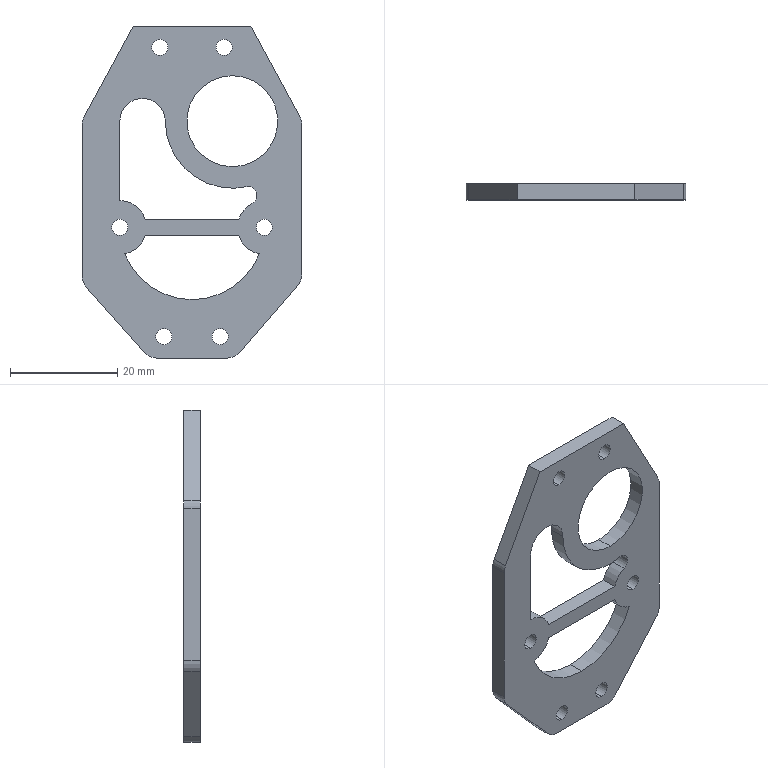Part | SolidWorks | features Extrusion 1, Fillet 1 | 1 solid | 43 faces | box 40.999 x 3 x 62 mm | volume 4212 mm3 | cylinder 30 | plane 13 | commonest cylinder face diameters 3 x12 6 x6 10 x4 17 x2 25 x2 27 x2
STEP:
#1=CARTESIAN_POINT('',(-4.98,3.,-17.786));
#2=VERTEX_POINT('',#1);
#3=CARTESIAN_POINT('',(7.52,3.,-30.28));
#4=VERTEX_POINT('',#3);
#5=CARTESIAN_POINT('',(7.52,3.,-17.78));
#6=DIRECTION('',(0.,-1.,0.));
#7=DIRECTION('',(0.,0.,1.));
#8=AXIS2_PLACEMENT_3D('',#5,#6,#7);
#9=CIRCLE('',#8,12.5);
#10=EDGE_CURVE('',#2,#4,#9,.T.);
#11=ORIENTED_EDGE('',*,*,#10,.T.);
#12=CARTESIAN_POINT('',(7.52,0.,-30.28));
#13=VERTEX_POINT('',#12);
#14=CARTESIAN_POINT('',(7.52,3.,-30.28));
#15=DIRECTION('',(0.,-1.,0.));
#16=VECTOR('',#15,1000.);
#17=LINE('',#14,#16);
#18=EDGE_CURVE('',#4,#13,#17,.T.);
#19=ORIENTED_EDGE('',*,*,#18,.T.);
#20=CARTESIAN_POINT('',(-4.98,0.,-17.786));
#21=VERTEX_POINT('',#20);
#22=CARTESIAN_POINT('',(7.52,0.,-17.78));
#23=DIRECTION('',(0.,-1.,0.));
#24=DIRECTION('',(0.,0.,1.));
#25=AXIS2_PLACEMENT_3D('',#22,#23,#24);
#26=CIRCLE('',#25,12.5);
#27=EDGE_CURVE('',#21,#13,#26,.T.);
#28=ORIENTED_EDGE('',*,*,#27,.F.);
#29=CARTESIAN_POINT('',(-4.98,3.,-17.786));
#30=DIRECTION('',(0.,-1.,0.));
#31=VECTOR('',#30,1000.);
#32=LINE('',#29,#31);
#33=EDGE_CURVE('',#2,#21,#32,.T.);
#34=ORIENTED_EDGE('',*,*,#33,.F.);
#35=EDGE_LOOP('',(#11,#19,#28,#34));
#36=FACE_OUTER_BOUND('',#35,.T.);
#37=CARTESIAN_POINT('',(7.52,3.,-17.78));
#38=DIRECTION('',(0.,-1.,0.));
#39=DIRECTION('',(0.,0.,-1.));
#40=AXIS2_PLACEMENT_3D('',#37,#38,#39);
#41=CYLINDRICAL_SURFACE('',#40,12.5);
#42=ADVANCED_FACE('',(#36),#41,.T.);
#43=CARTESIAN_POINT('',(12.574,3.,-42.519));
#44=VERTEX_POINT('',#43);
#45=CARTESIAN_POINT('',(0.,3.,-51.105));
#46=VERTEX_POINT('',#45);
#47=CARTESIAN_POINT('',(0.,3.,-37.605));
#48=DIRECTION('',(0.,1.,0.));
#49=DIRECTION('',(0.,0.,1.));
#50=AXIS2_PLACEMENT_3D('',#47,#48,#49);
#51=CIRCLE('',#50,13.5);
#52=EDGE_CURVE('',#44,#46,#51,.T.);
#53=ORIENTED_EDGE('',*,*,#52,.T.);
#54=CARTESIAN_POINT('',(0.,0.,-51.105));
#55=VERTEX_POINT('',#54);
#56=CARTESIAN_POINT('',(0.,3.,-51.105));
#57=DIRECTION('',(0.,-1.,0.));
#58=VECTOR('',#57,1000.);
#59=LINE('',#56,#58);
#60=EDGE_CURVE('',#46,#55,#59,.T.);
#61=ORIENTED_EDGE('',*,*,#60,.T.);
#62=CARTESIAN_POINT('',(12.574,0.,-42.519));
#63=VERTEX_POINT('',#62);
#64=CARTESIAN_POINT('',(0.,0.,-37.605));
#65=DIRECTION('',(0.,1.,0.));
#66=DIRECTION('',(0.,0.,1.));
#67=AXIS2_PLACEMENT_3D('',#64,#65,#66);
#68=CIRCLE('',#67,13.5);
#69=EDGE_CURVE('',#63,#55,#68,.T.);
#70=ORIENTED_EDGE('',*,*,#69,.F.);
#71=CARTESIAN_POINT('',(12.574,3.,-42.519));
#72=DIRECTION('',(0.,-1.,0.));
#73=VECTOR('',#72,1000.);
#74=LINE('',#71,#73);
#75=EDGE_CURVE('',#44,#63,#74,.T.);
#76=ORIENTED_EDGE('',*,*,#75,.F.);
#77=EDGE_LOOP('',(#53,#61,#70,#76));
#78=FACE_OUTER_BOUND('',#77,.T.);
#79=CARTESIAN_POINT('',(0.,3.,-37.605));
#80=DIRECTION('',(0.,-1.,0.));
#81=DIRECTION('',(0.,0.,-1.));
#82=AXIS2_PLACEMENT_3D('',#79,#80,#81);
#83=CYLINDRICAL_SURFACE('',#82,13.5);
#84=ADVANCED_FACE('',(#78),#83,.F.);
#85=CARTESIAN_POINT('',(13.5,3.,-39.105));
#86=VERTEX_POINT('',#85);
#87=CARTESIAN_POINT('',(13.5,3.,-36.105));
#88=VERTEX_POINT('',#87);
#89=CARTESIAN_POINT('',(13.5,3.,-37.605));
#90=DIRECTION('',(0.,1.,0.));
#91=DIRECTION('',(0.,0.,1.));
#92=AXIS2_PLACEMENT_3D('',#89,#90,#91);
#93=CIRCLE('',#92,1.5);
#94=EDGE_CURVE('',#86,#88,#93,.T.);
#95=ORIENTED_EDGE('',*,*,#94,.T.);
#96=CARTESIAN_POINT('',(13.5,0.,-36.105));
#97=VERTEX_POINT('',#96);
#98=CARTESIAN_POINT('',(13.5,3.,-36.105));
#99=DIRECTION('',(0.,-1.,0.));
#100=VECTOR('',#99,1000.);
#101=LINE('',#98,#100);
#102=EDGE_CURVE('',#88,#97,#101,.T.);
#103=ORIENTED_EDGE('',*,*,#102,.T.);
#104=CARTESIAN_POINT('',(13.5,0.,-39.105));
#105=VERTEX_POINT('',#104);
#106=CARTESIAN_POINT('',(13.5,0.,-37.605));
#107=DIRECTION('',(0.,1.,0.));
#108=DIRECTION('',(0.,0.,1.));
#109=AXIS2_PLACEMENT_3D('',#106,#107,#108);
#110=CIRCLE('',#109,1.5);
#111=EDGE_CURVE('',#105,#97,#110,.T.);
#112=ORIENTED_EDGE('',*,*,#111,.F.);
#113=CARTESIAN_POINT('',(13.5,3.,-39.105));
#114=DIRECTION('',(0.,-1.,0.));
#115=VECTOR('',#114,1000.);
#116=LINE('',#113,#115);
#117=EDGE_CURVE('',#86,#105,#116,.T.);
#118=ORIENTED_EDGE('',*,*,#117,.F.);
#119=EDGE_LOOP('',(#95,#103,#112,#118));
#120=FACE_OUTER_BOUND('',#119,.T.);
#121=CARTESIAN_POINT('',(13.5,3.,-37.605));
#122=DIRECTION('',(0.,-1.,0.));
#123=DIRECTION('',(0.,0.,-1.));
#124=AXIS2_PLACEMENT_3D('',#121,#122,#123);
#125=CYLINDRICAL_SURFACE('',#124,1.5);
#126=ADVANCED_FACE('',(#120),#125,.F.);
#127=CARTESIAN_POINT('',(-13.5,3.,-39.105));
#128=VERTEX_POINT('',#127);
#129=CARTESIAN_POINT('',(-13.5,3.,-36.105));
#130=VERTEX_POINT('',#129);
#131=CARTESIAN_POINT('',(-13.5,3.,-37.605));
#132=DIRECTION('',(0.,1.,0.));
#133=DIRECTION('',(0.,0.,1.));
#134=AXIS2_PLACEMENT_3D('',#131,#132,#133);
#135=CIRCLE('',#134,1.5);
#136=EDGE_CURVE('',#128,#130,#135,.T.);
#137=ORIENTED_EDGE('',*,*,#136,.T.);
#138=CARTESIAN_POINT('',(-13.5,0.,-36.105));
#139=VERTEX_POINT('',#138);
#140=CARTESIAN_POINT('',(-13.5,3.,-36.105));
#141=DIRECTION('',(0.,-1.,0.));
#142=VECTOR('',#141,1000.);
#143=LINE('',#140,#142);
#144=EDGE_CURVE('',#130,#139,#143,.T.);
#145=ORIENTED_EDGE('',*,*,#144,.T.);
#146=CARTESIAN_POINT('',(-13.5,0.,-39.105));
#147=VERTEX_POINT('',#146);
#148=CARTESIAN_POINT('',(-13.5,0.,-37.605));
#149=DIRECTION('',(0.,1.,0.));
#150=DIRECTION('',(0.,0.,1.));
#151=AXIS2_PLACEMENT_3D('',#148,#149,#150);
#152=CIRCLE('',#151,1.5);
#153=EDGE_CURVE('',#147,#139,#152,.T.);
#154=ORIENTED_EDGE('',*,*,#153,.F.);
#155=CARTESIAN_POINT('',(-13.5,3.,-39.105));
#156=DIRECTION('',(0.,-1.,0.));
#157=VECTOR('',#156,1000.);
#158=LINE('',#155,#157);
#159=EDGE_CURVE('',#128,#147,#158,.T.);
#160=ORIENTED_EDGE('',*,*,#159,.F.);
#161=EDGE_LOOP('',(#137,#145,#154,#160));
#162=FACE_OUTER_BOUND('',#161,.T.);
#163=CARTESIAN_POINT('',(-13.5,3.,-37.605));
#164=DIRECTION('',(0.,-1.,0.));
#165=DIRECTION('',(0.,0.,-1.));
#166=AXIS2_PLACEMENT_3D('',#163,#164,#165);
#167=CYLINDRICAL_SURFACE('',#166,1.5);
#168=ADVANCED_FACE('',(#162),#167,.F.);
#169=CARTESIAN_POINT('',(5.25,3.,-59.5));
#170=VERTEX_POINT('',#169);
#171=CARTESIAN_POINT('',(5.25,3.,-56.5));
#172=VERTEX_POINT('',#171);
#173=CARTESIAN_POINT('',(5.25,3.,-58.));
#174=DIRECTION('',(0.,1.,0.));
#175=DIRECTION('',(0.,0.,1.));
#176=AXIS2_PLACEMENT_3D('',#173,#174,#175);
#177=CIRCLE('',#176,1.5);
#178=EDGE_CURVE('',#170,#172,#177,.T.);
#179=ORIENTED_EDGE('',*,*,#178,.T.);
#180=CARTESIAN_POINT('',(5.25,0.,-56.5));
#181=VERTEX_POINT('',#180);
#182=CARTESIAN_POINT('',(5.25,3.,-56.5));
#183=DIRECTION('',(0.,-1.,0.));
#184=VECTOR('',#183,1000.);
#185=LINE('',#182,#184);
#186=EDGE_CURVE('',#172,#181,#185,.T.);
#187=ORIENTED_EDGE('',*,*,#186,.T.);
#188=CARTESIAN_POINT('',(5.25,0.,-59.5));
#189=VERTEX_POINT('',#188);
#190=CARTESIAN_POINT('',(5.25,0.,-58.));
#191=DIRECTION('',(0.,1.,0.));
#192=DIRECTION('',(0.,0.,1.));
#193=AXIS2_PLACEMENT_3D('',#190,#191,#192);
#194=CIRCLE('',#193,1.5);
#195=EDGE_CURVE('',#189,#181,#194,.T.);
#196=ORIENTED_EDGE('',*,*,#195,.F.);
#197=CARTESIAN_POINT('',(5.25,3.,-59.5));
#198=DIRECTION('',(0.,-1.,0.));
#199=VECTOR('',#198,1000.);
#200=LINE('',#197,#199);
#201=EDGE_CURVE('',#170,#189,#200,.T.);
#202=ORIENTED_EDGE('',*,*,#201,.F.);
#203=EDGE_LOOP('',(#179,#187,#196,#202));
#204=FACE_OUTER_BOUND('',#203,.T.);
#205=CARTESIAN_POINT('',(5.25,3.,-58.));
#206=DIRECTION('',(0.,-1.,0.));
#207=DIRECTION('',(0.,0.,-1.));
#208=AXIS2_PLACEMENT_3D('',#205,#206,#207);
#209=CYLINDRICAL_SURFACE('',#208,1.5);
#210=ADVANCED_FACE('',(#204),#209,.F.);
#211=CARTESIAN_POINT('',(-5.25,3.,-59.5));
#212=VERTEX_POINT('',#211);
#213=CARTESIAN_POINT('',(-5.25,3.,-56.5));
#214=VERTEX_POINT('',#213);
#215=CARTESIAN_POINT('',(-5.25,3.,-58.));
#216=DIRECTION('',(0.,1.,0.));
#217=DIRECTION('',(0.,0.,1.));
#218=AXIS2_PLACEMENT_3D('',#215,#216,#217);
#219=CIRCLE('',#218,1.5);
#220=EDGE_CURVE('',#212,#214,#219,.T.);
#221=ORIENTED_EDGE('',*,*,#220,.T.);
#222=CARTESIAN_POINT('',(-5.25,0.,-56.5));
#223=VERTEX_POINT('',#222);
#224=CARTESIAN_POINT('',(-5.25,3.,-56.5));
#225=DIRECTION('',(0.,-1.,0.));
#226=VECTOR('',#225,1000.);
#227=LINE('',#224,#226);
#228=EDGE_CURVE('',#214,#223,#227,.T.);
#229=ORIENTED_EDGE('',*,*,#228,.T.);
#230=CARTESIAN_POINT('',(-5.25,0.,-59.5));
#231=VERTEX_POINT('',#230);
#232=CARTESIAN_POINT('',(-5.25,0.,-58.));
#233=DIRECTION('',(0.,1.,0.));
#234=DIRECTION('',(0.,0.,1.));
#235=AXIS2_PLACEMENT_3D('',#232,#233,#234);
#236=CIRCLE('',#235,1.5);
#237=EDGE_CURVE('',#231,#223,#236,.T.);
#238=ORIENTED_EDGE('',*,*,#237,.F.);
#239=CARTESIAN_POINT('',(-5.25,3.,-59.5));
#240=DIRECTION('',(0.,-1.,0.));
#241=VECTOR('',#240,1000.);
#242=LINE('',#239,#241);
#243=EDGE_CURVE('',#212,#231,#242,.T.);
#244=ORIENTED_EDGE('',*,*,#243,.F.);
#245=EDGE_LOOP('',(#221,#229,#238,#244));
#246=FACE_OUTER_BOUND('',#245,.T.);
#247=CARTESIAN_POINT('',(-5.25,3.,-58.));
#248=DIRECTION('',(0.,-1.,0.));
#249=DIRECTION('',(0.,0.,-1.));
#250=AXIS2_PLACEMENT_3D('',#247,#248,#249);
#251=CYLINDRICAL_SURFACE('',#250,1.5);
#252=ADVANCED_FACE('',(#246),#251,.F.);
#253=CARTESIAN_POINT('',(-6.,3.,-5.5));
#254=VERTEX_POINT('',#253);
#255=CARTESIAN_POINT('',(-6.,3.,-2.5));
#256=VERTEX_POINT('',#255);
#257=CARTESIAN_POINT('',(-6.,3.,-4.));
#258=DIRECTION('',(0.,1.,0.));
#259=DIRECTION('',(0.,0.,-1.));
#260=AXIS2_PLACEMENT_3D('',#257,#258,#259);
#261=CIRCLE('',#260,1.5);
#262=EDGE_CURVE('',#254,#256,#261,.T.);
#263=ORIENTED_EDGE('',*,*,#262,.T.);
#264=CARTESIAN_POINT('',(-6.,0.,-2.5));
#265=VERTEX_POINT('',#264);
#266=CARTESIAN_POINT('',(-6.,3.,-2.5));
#267=DIRECTION('',(0.,-1.,0.));
#268=VECTOR('',#267,1000.);
#269=LINE('',#266,#268);
#270=EDGE_CURVE('',#256,#265,#269,.T.);
#271=ORIENTED_EDGE('',*,*,#270,.T.);
#272=CARTESIAN_POINT('',(-6.,0.,-5.5));
#273=VERTEX_POINT('',#272);
#274=CARTESIAN_POINT('',(-6.,0.,-4.));
#275=DIRECTION('',(0.,1.,0.));
#276=DIRECTION('',(0.,0.,-1.));
#277=AXIS2_PLACEMENT_3D('',#274,#275,#276);
#278=CIRCLE('',#277,1.5);
#279=EDGE_CURVE('',#273,#265,#278,.T.);
#280=ORIENTED_EDGE('',*,*,#279,.F.);
#281=CARTESIAN_POINT('',(-6.,3.,-5.5));
#282=DIRECTION('',(0.,-1.,0.));
#283=VECTOR('',#282,1000.);
#284=LINE('',#281,#283);
#285=EDGE_CURVE('',#254,#273,#284,.T.);
#286=ORIENTED_EDGE('',*,*,#285,.F.);
#287=EDGE_LOOP('',(#263,#271,#280,#286));
#288=FACE_OUTER_BOUND('',#287,.T.);
#289=CARTESIAN_POINT('',(-6.,3.,-4.));
#290=DIRECTION('',(0.,-1.,0.));
#291=DIRECTION('',(0.,0.,-1.));
#292=AXIS2_PLACEMENT_3D('',#289,#290,#291);
#293=CYLINDRICAL_SURFACE('',#292,1.5);
#294=ADVANCED_FACE('',(#288),#293,.F.);
#295=CARTESIAN_POINT('',(6.,3.,-5.5));
#296=VERTEX_POINT('',#295);
#297=CARTESIAN_POINT('',(6.,3.,-2.5));
#298=VERTEX_POINT('',#297);
#299=CARTESIAN_POINT('',(6.,3.,-4.));
#300=DIRECTION('',(0.,1.,0.));
#301=DIRECTION('',(0.,0.,1.));
#302=AXIS2_PLACEMENT_3D('',#299,#300,#301);
#303=CIRCLE('',#302,1.5);
#304=EDGE_CURVE('',#296,#298,#303,.T.);
#305=ORIENTED_EDGE('',*,*,#304,.T.);
#306=CARTESIAN_POINT('',(6.,0.,-2.5));
#307=VERTEX_POINT('',#306);
#308=CARTESIAN_POINT('',(6.,3.,-2.5));
#309=DIRECTION('',(0.,-1.,0.));
#310=VECTOR('',#309,1000.);
#311=LINE('',#308,#310);
#312=EDGE_CURVE('',#298,#307,#311,.T.);
#313=ORIENTED_EDGE('',*,*,#312,.T.);
#314=CARTESIAN_POINT('',(6.,0.,-5.5));
#315=VERTEX_POINT('',#314);
#316=CARTESIAN_POINT('',(6.,0.,-4.));
#317=DIRECTION('',(0.,1.,0.));
#318=DIRECTION('',(0.,0.,1.));
#319=AXIS2_PLACEMENT_3D('',#316,#317,#318);
#320=CIRCLE('',#319,1.5);
#321=EDGE_CURVE('',#315,#307,#320,.T.);
#322=ORIENTED_EDGE('',*,*,#321,.F.);
#323=CARTESIAN_POINT('',(6.,3.,-5.5));
#324=DIRECTION('',(0.,-1.,0.));
#325=VECTOR('',#324,1000.);
#326=LINE('',#323,#325);
#327=EDGE_CURVE('',#296,#315,#326,.T.);
#328=ORIENTED_EDGE('',*,*,#327,.F.);
#329=EDGE_LOOP('',(#305,#313,#322,#328));
#330=FACE_OUTER_BOUND('',#329,.T.);
#331=CARTESIAN_POINT('',(6.,3.,-4.));
#332=DIRECTION('',(0.,-1.,0.));
#333=DIRECTION('',(0.,0.,-1.));
#334=AXIS2_PLACEMENT_3D('',#331,#332,#333);
#335=CYLINDRICAL_SURFACE('',#334,1.5);
#336=ADVANCED_FACE('',(#330),#335,.F.);
#337=CARTESIAN_POINT('',(7.52,3.,-26.28));
#338=VERTEX_POINT('',#337);
#339=CARTESIAN_POINT('',(7.52,3.,-9.28));
#340=VERTEX_POINT('',#339);
#341=CARTESIAN_POINT('',(7.52,3.,-17.78));
#342=DIRECTION('',(0.,1.,0.));
#343=DIRECTION('',(0.,0.,1.));
#344=AXIS2_PLACEMENT_3D('',#341,#342,#343);
#345=CIRCLE('',#344,8.5);
#346=EDGE_CURVE('',#338,#340,#345,.T.);
#347=ORIENTED_EDGE('',*,*,#346,.T.);
#348=CARTESIAN_POINT('',(7.52,0.,-9.28));
#349=VERTEX_POINT('',#348);
#350=CARTESIAN_POINT('',(7.52,3.,-9.28));
#351=DIRECTION('',(0.,-1.,0.));
#352=VECTOR('',#351,1000.);
#353=LINE('',#350,#352);
#354=EDGE_CURVE('',#340,#349,#353,.T.);
#355=ORIENTED_EDGE('',*,*,#354,.T.);
#356=CARTESIAN_POINT('',(7.52,0.,-26.28));
#357=VERTEX_POINT('',#356);
#358=CARTESIAN_POINT('',(7.52,0.,-17.78));
#359=DIRECTION('',(0.,1.,0.));
#360=DIRECTION('',(0.,0.,1.));
#361=AXIS2_PLACEMENT_3D('',#358,#359,#360);
#362=CIRCLE('',#361,8.5);
#363=EDGE_CURVE('',#357,#349,#362,.T.);
#364=ORIENTED_EDGE('',*,*,#363,.F.);
#365=CARTESIAN_POINT('',(7.52,3.,-26.28));
#366=DIRECTION('',(0.,-1.,0.));
#367=VECTOR('',#366,1000.);
#368=LINE('',#365,#367);
#369=EDGE_CURVE('',#338,#357,#368,.T.);
#370=ORIENTED_EDGE('',*,*,#369,.F.);
#371=EDGE_LOOP('',(#347,#355,#364,#370));
#372=FACE_OUTER_BOUND('',#371,.T.);
#373=CARTESIAN_POINT('',(7.52,3.,-17.78));
#374=DIRECTION('',(0.,-1.,0.));
#375=DIRECTION('',(0.,0.,-1.));
#376=AXIS2_PLACEMENT_3D('',#373,#374,#375);
#377=CYLINDRICAL_SURFACE('',#376,8.5);
#378=ADVANCED_FACE('',(#372),#377,.F.);
#379=ORIENTED_EDGE('',*,*,#52,.F.);
#380=CARTESIAN_POINT('',(8.73,3.,-39.105));
#381=VERTEX_POINT('',#380);
#382=CARTESIAN_POINT('',(13.5,3.,-37.605));
#383=DIRECTION('',(0.,-1.,0.));
#384=DIRECTION('',(0.,0.,1.));
#385=AXIS2_PLACEMENT_3D('',#382,#383,#384);
#386=CIRCLE('',#385,5.);
#387=EDGE_CURVE('',#381,#44,#386,.T.);
#388=ORIENTED_EDGE('',*,*,#387,.F.);
#389=CARTESIAN_POINT('',(-8.73,3.,-39.105));
#390=VERTEX_POINT('',#389);
#391=CARTESIAN_POINT('',(-8.73,3.,-39.105));
#392=DIRECTION('',(1.,0.,0.));
#393=VECTOR('',#392,1000.);
#394=LINE('',#391,#393);
#395=EDGE_CURVE('',#390,#381,#394,.T.);
#396=ORIENTED_EDGE('',*,*,#395,.F.);
#397=CARTESIAN_POINT('',(-12.574,3.,-42.519));
#398=VERTEX_POINT('',#397);
#399=CARTESIAN_POINT('',(-13.5,3.,-37.605));
#400=DIRECTION('',(0.,-1.,0.));
#401=DIRECTION('',(0.,0.,1.));
#402=AXIS2_PLACEMENT_3D('',#399,#400,#401);
#403=CIRCLE('',#402,5.);
#404=EDGE_CURVE('',#398,#390,#403,.T.);
#405=ORIENTED_EDGE('',*,*,#404,.F.);
#406=CARTESIAN_POINT('',(0.,3.,-37.605));
#407=DIRECTION('',(0.,1.,0.));
#408=DIRECTION('',(0.,0.,1.));
#409=AXIS2_PLACEMENT_3D('',#406,#407,#408);
#410=CIRCLE('',#409,13.5);
#411=EDGE_CURVE('',#46,#398,#410,.T.);
#412=ORIENTED_EDGE('',*,*,#411,.F.);
#413=EDGE_LOOP('',(#379,#388,#396,#405,#412));
#414=FACE_BOUND('',#413,.T.);
#415=CARTESIAN_POINT('',(19.756,3.,-48.451));
#416=VERTEX_POINT('',#415);
#417=CARTESIAN_POINT('',(8.897,3.,-60.966));
#418=VERTEX_POINT('',#417);
#419=CARTESIAN_POINT('',(20.49,3.,-47.605));
#420=DIRECTION('',(-0.6554,0.,-0.7553));
#421=VECTOR('',#420,1000.);
#422=LINE('',#419,#421);
#423=EDGE_CURVE('',#416,#418,#422,.T.);
#424=ORIENTED_EDGE('',*,*,#423,.T.);
#425=CARTESIAN_POINT('',(6.631,3.,-62.));
#426=VERTEX_POINT('',#425);
#427=CARTESIAN_POINT('',(6.631,3.,-59.));
#428=DIRECTION('',(0.,1.,0.));
#429=DIRECTION('',(0.,0.,-1.));
#430=AXIS2_PLACEMENT_3D('',#427,#428,#429);
#431=CIRCLE('',#430,3.);
#432=EDGE_CURVE('',#418,#426,#431,.T.);
#433=ORIENTED_EDGE('',*,*,#432,.T.);
#434=CARTESIAN_POINT('',(-6.652,3.,-62.));
#435=VERTEX_POINT('',#434);
#436=CARTESIAN_POINT('',(-8.,3.,-62.));
#437=DIRECTION('',(-1.,0.,0.));
#438=VECTOR('',#437,1000.);
#439=LINE('',#436,#438);
#440=EDGE_CURVE('',#426,#435,#439,.T.);
#441=ORIENTED_EDGE('',*,*,#440,.T.);
#442=CARTESIAN_POINT('',(-8.895,3.,-60.992));
#443=VERTEX_POINT('',#442);
#444=CARTESIAN_POINT('',(-6.652,3.,-59.));
#445=DIRECTION('',(0.,1.,0.));
#446=DIRECTION('',(0.,0.,-1.));
#447=AXIS2_PLACEMENT_3D('',#444,#445,#446);
#448=CIRCLE('',#447,3.);
#449=EDGE_CURVE('',#435,#443,#448,.T.);
#450=ORIENTED_EDGE('',*,*,#449,.T.);
#451=CARTESIAN_POINT('',(-19.753,3.,-48.762));
#452=VERTEX_POINT('',#451);
#453=CARTESIAN_POINT('',(-20.509,3.,-47.91));
#454=DIRECTION('',(-0.6639,0.,0.7478));
#455=VECTOR('',#454,1000.);
#456=LINE('',#453,#455);
#457=EDGE_CURVE('',#443,#452,#456,.T.);
#458=ORIENTED_EDGE('',*,*,#457,.T.);
#459=CARTESIAN_POINT('',(-20.509,3.,-46.771));
#460=VERTEX_POINT('',#459);
#461=CARTESIAN_POINT('',(-17.509,3.,-46.771));
#462=DIRECTION('',(0.,1.,0.));
#463=DIRECTION('',(0.,0.,-1.));
#464=AXIS2_PLACEMENT_3D('',#461,#462,#463);
#465=CIRCLE('',#464,3.);
#466=EDGE_CURVE('',#452,#460,#465,.T.);
#467=ORIENTED_EDGE('',*,*,#466,.T.);
#468=CARTESIAN_POINT('',(-20.509,3.,-18.369));
#469=VERTEX_POINT('',#468);
#470=CARTESIAN_POINT('',(-20.509,3.,-17.611));
#471=DIRECTION('',(0.,0.,1.));
#472=VECTOR('',#471,1000.);
#473=LINE('',#470,#472);
#474=EDGE_CURVE('',#460,#469,#473,.T.);
#475=ORIENTED_EDGE('',*,*,#474,.T.);
#476=CARTESIAN_POINT('',(-20.149,3.,-16.944));
#477=VERTEX_POINT('',#476);
#478=CARTESIAN_POINT('',(-17.509,3.,-18.369));
#479=DIRECTION('',(0.,1.,0.));
#480=DIRECTION('',(0.,0.,-1.));
#481=AXIS2_PLACEMENT_3D('',#478,#479,#480);
#482=CIRCLE('',#481,3.);
#483=EDGE_CURVE('',#469,#477,#482,.T.);
#484=ORIENTED_EDGE('',*,*,#483,.T.);
#485=CARTESIAN_POINT('',(-11.,3.,0.));
#486=VERTEX_POINT('',#485);
#487=CARTESIAN_POINT('',(-11.,3.,0.));
#488=DIRECTION('',(0.4751,0.,0.8799));
#489=VECTOR('',#488,1000.);
#490=LINE('',#487,#489);
#491=EDGE_CURVE('',#477,#486,#490,.T.);
#492=ORIENTED_EDGE('',*,*,#491,.T.);
#493=CARTESIAN_POINT('',(11.,3.,0.));
#494=VERTEX_POINT('',#493);
#495=CARTESIAN_POINT('',(-11.,3.,0.));
#496=DIRECTION('',(1.,0.,0.));
#497=VECTOR('',#496,1000.);
#498=LINE('',#495,#497);
#499=EDGE_CURVE('',#486,#494,#498,.T.);
#500=ORIENTED_EDGE('',*,*,#499,.T.);
#501=CARTESIAN_POINT('',(20.13,3.,-16.939));
#502=VERTEX_POINT('',#501);
#503=CARTESIAN_POINT('',(11.,3.,0.));
#504=DIRECTION('',(0.4745,0.,-0.8803));
#505=VECTOR('',#504,1000.);
#506=LINE('',#503,#505);
#507=EDGE_CURVE('',#494,#502,#506,.T.);
#508=ORIENTED_EDGE('',*,*,#507,.T.);
#509=CARTESIAN_POINT('',(20.49,3.,-18.362));
#510=VERTEX_POINT('',#509);
#511=CARTESIAN_POINT('',(17.49,3.,-18.362));
#512=DIRECTION('',(0.,1.,0.));
#513=DIRECTION('',(0.,0.,-1.));
#514=AXIS2_PLACEMENT_3D('',#511,#512,#513);
#515=CIRCLE('',#514,3.);
#516=EDGE_CURVE('',#502,#510,#515,.T.);
#517=ORIENTED_EDGE('',*,*,#516,.T.);
#518=CARTESIAN_POINT('',(20.49,3.,-46.485));
#519=VERTEX_POINT('',#518);
#520=CARTESIAN_POINT('',(20.49,3.,-17.605));
#521=DIRECTION('',(0.,0.,-1.));
#522=VECTOR('',#521,1000.);
#523=LINE('',#520,#522);
#524=EDGE_CURVE('',#510,#519,#523,.T.);
#525=ORIENTED_EDGE('',*,*,#524,.T.);
#526=CARTESIAN_POINT('',(17.49,3.,-46.485));
#527=DIRECTION('',(0.,1.,0.));
#528=DIRECTION('',(0.,0.,-1.));
#529=AXIS2_PLACEMENT_3D('',#526,#527,#528);
#530=CIRCLE('',#529,3.);
#531=EDGE_CURVE('',#519,#416,#530,.T.);
#532=ORIENTED_EDGE('',*,*,#531,.T.);
#533=EDGE_LOOP('',(#424,#433,#441,#450,#458,#467,#475,#484,#492,#500,#508,#517,#525,#532));
#534=FACE_OUTER_BOUND('',#533,.T.);
#535=ORIENTED_EDGE('',*,*,#346,.F.);
#536=CARTESIAN_POINT('',(7.52,3.,-17.78));
#537=DIRECTION('',(0.,1.,0.));
#538=DIRECTION('',(0.,0.,1.));
#539=AXIS2_PLACEMENT_3D('',#536,#537,#538);
#540=CIRCLE('',#539,8.5);
#541=EDGE_CURVE('',#340,#338,#540,.T.);
#542=ORIENTED_EDGE('',*,*,#541,.F.);
#543=EDGE_LOOP('',(#535,#542));
#544=FACE_BOUND('',#543,.T.);
#545=ORIENTED_EDGE('',*,*,#304,.F.);
#546=CARTESIAN_POINT('',(6.,3.,-4.));
#547=DIRECTION('',(0.,1.,0.));
#548=DIRECTION('',(0.,0.,1.));
#549=AXIS2_PLACEMENT_3D('',#546,#547,#548);
#550=CIRCLE('',#549,1.5);
#551=EDGE_CURVE('',#298,#296,#550,.T.);
#552=ORIENTED_EDGE('',*,*,#551,.F.);
#553=EDGE_LOOP('',(#545,#552));
#554=FACE_BOUND('',#553,.T.);
#555=ORIENTED_EDGE('',*,*,#262,.F.);
#556=CARTESIAN_POINT('',(-6.,3.,-4.));
#557=DIRECTION('',(0.,1.,0.));
#558=DIRECTION('',(0.,0.,-1.));
#559=AXIS2_PLACEMENT_3D('',#556,#557,#558);
#560=CIRCLE('',#559,1.5);
#561=EDGE_CURVE('',#256,#254,#560,.T.);
#562=ORIENTED_EDGE('',*,*,#561,.F.);
#563=EDGE_LOOP('',(#555,#562));
#564=FACE_BOUND('',#563,.T.);
#565=ORIENTED_EDGE('',*,*,#220,.F.);
#566=CARTESIAN_POINT('',(-5.25,3.,-58.));
#567=DIRECTION('',(0.,1.,0.));
#568=DIRECTION('',(0.,0.,1.));
#569=AXIS2_PLACEMENT_3D('',#566,#567,#568);
#570=CIRCLE('',#569,1.5);
#571=EDGE_CURVE('',#214,#212,#570,.T.);
#572=ORIENTED_EDGE('',*,*,#571,.F.);
#573=EDGE_LOOP('',(#565,#572));
#574=FACE_BOUND('',#573,.T.);
#575=ORIENTED_EDGE('',*,*,#178,.F.);
#576=CARTESIAN_POINT('',(5.25,3.,-58.));
#577=DIRECTION('',(0.,1.,0.));
#578=DIRECTION('',(0.,0.,1.));
#579=AXIS2_PLACEMENT_3D('',#576,#577,#578);
#580=CIRCLE('',#579,1.5);
#581=EDGE_CURVE('',#172,#170,#580,.T.);
#582=ORIENTED_EDGE('',*,*,#581,.F.);
#583=EDGE_LOOP('',(#575,#582));
#584=FACE_BOUND('',#583,.T.);
#585=ORIENTED_EDGE('',*,*,#136,.F.);
#586=CARTESIAN_POINT('',(-13.5,3.,-37.605));
#587=DIRECTION('',(0.,1.,0.));
#588=DIRECTION('',(0.,0.,1.));
#589=AXIS2_PLACEMENT_3D('',#586,#587,#588);
#590=CIRCLE('',#589,1.5);
#591=EDGE_CURVE('',#130,#128,#590,.T.);
#592=ORIENTED_EDGE('',*,*,#591,.F.);
#593=EDGE_LOOP('',(#585,#592));
#594=FACE_BOUND('',#593,.T.);
#595=ORIENTED_EDGE('',*,*,#94,.F.);
#596=CARTESIAN_POINT('',(13.5,3.,-37.605));
#597=DIRECTION('',(0.,1.,0.));
#598=DIRECTION('',(0.,0.,1.));
#599=AXIS2_PLACEMENT_3D('',#596,#597,#598);
#600=CIRCLE('',#599,1.5);
#601=EDGE_CURVE('',#88,#86,#600,.T.);
#602=ORIENTED_EDGE('',*,*,#601,.F.);
#603=EDGE_LOOP('',(#595,#602));
#604=FACE_BOUND('',#603,.T.);
#605=CARTESIAN_POINT('',(10.063,3.,-30.019));
#606=VERTEX_POINT('',#605);
#607=CARTESIAN_POINT('',(11.188,3.,-33.172));
#608=VERTEX_POINT('',#607);
#609=CARTESIAN_POINT('',(10.407,3.,-31.673));
#610=DIRECTION('',(0.,1.,0.));
#611=DIRECTION('',(0.,0.,1.));
#612=AXIS2_PLACEMENT_3D('',#609,#610,#611);
#613=CIRCLE('',#612,1.69);
#614=EDGE_CURVE('',#606,#608,#613,.T.);
#615=ORIENTED_EDGE('',*,*,#614,.F.);
#616=CARTESIAN_POINT('',(7.52,3.,-17.78));
#617=DIRECTION('',(0.,-1.,0.));
#618=DIRECTION('',(0.,0.,1.));
#619=AXIS2_PLACEMENT_3D('',#616,#617,#618);
#620=CIRCLE('',#619,12.5);
#621=EDGE_CURVE('',#4,#606,#620,.T.);
#622=ORIENTED_EDGE('',*,*,#621,.F.);
#623=ORIENTED_EDGE('',*,*,#10,.F.);
#624=CARTESIAN_POINT('',(-13.5,3.,-17.788));
#625=VERTEX_POINT('',#624);
#626=CARTESIAN_POINT('',(-9.24,3.,-17.788));
#627=DIRECTION('',(0.,1.,0.));
#628=DIRECTION('',(0.,0.,1.));
#629=AXIS2_PLACEMENT_3D('',#626,#627,#628);
#630=CIRCLE('',#629,4.26);
#631=EDGE_CURVE('',#625,#2,#630,.T.);
#632=ORIENTED_EDGE('',*,*,#631,.F.);
#633=CARTESIAN_POINT('',(-13.5,3.,-32.605));
#634=VERTEX_POINT('',#633);
#635=CARTESIAN_POINT('',(-13.5,3.,-32.605));
#636=DIRECTION('',(0.,0.,1.));
#637=VECTOR('',#636,1000.);
#638=LINE('',#635,#637);
#639=EDGE_CURVE('',#634,#625,#638,.T.);
#640=ORIENTED_EDGE('',*,*,#639,.F.);
#641=CARTESIAN_POINT('',(-8.73,3.,-36.105));
#642=VERTEX_POINT('',#641);
#643=CARTESIAN_POINT('',(-13.5,3.,-37.605));
#644=DIRECTION('',(0.,-1.,0.));
#645=DIRECTION('',(0.,0.,1.));
#646=AXIS2_PLACEMENT_3D('',#643,#644,#645);
#647=CIRCLE('',#646,5.);
#648=EDGE_CURVE('',#642,#634,#647,.T.);
#649=ORIENTED_EDGE('',*,*,#648,.F.);
#650=CARTESIAN_POINT('',(8.73,3.,-36.105));
#651=VERTEX_POINT('',#650);
#652=CARTESIAN_POINT('',(-8.73,3.,-36.105));
#653=DIRECTION('',(-1.,0.,0.));
#654=VECTOR('',#653,1000.);
#655=LINE('',#652,#654);
#656=EDGE_CURVE('',#651,#642,#655,.T.);
#657=ORIENTED_EDGE('',*,*,#656,.F.);
#658=CARTESIAN_POINT('',(13.5,3.,-37.605));
#659=DIRECTION('',(0.,-1.,0.));
#660=DIRECTION('',(0.,0.,1.));
#661=AXIS2_PLACEMENT_3D('',#658,#659,#660);
#662=CIRCLE('',#661,5.);
#663=EDGE_CURVE('',#608,#651,#662,.T.);
#664=ORIENTED_EDGE('',*,*,#663,.F.);
#665=EDGE_LOOP('',(#615,#622,#623,#632,#640,#649,#657,#664));
#666=FACE_BOUND('',#665,.T.);
#667=CARTESIAN_POINT('',(0.,3.,0.));
#668=DIRECTION('',(0.,-1.,0.));
#669=DIRECTION('',(0.,0.,-1.));
#670=AXIS2_PLACEMENT_3D('',#667,#668,#669);
#671=PLANE('',#670);
#672=ADVANCED_FACE('',(#414,#534,#544,#554,#564,#574,#584,#594,#604,#666),#671,.F.);
#673=ORIENTED_EDGE('',*,*,#153,.T.);
#674=CARTESIAN_POINT('',(-13.5,0.,-37.605));
#675=DIRECTION('',(0.,1.,0.));
#676=DIRECTION('',(0.,0.,1.));
#677=AXIS2_PLACEMENT_3D('',#674,#675,#676);
#678=CIRCLE('',#677,1.5);
#679=EDGE_CURVE('',#139,#147,#678,.T.);
#680=ORIENTED_EDGE('',*,*,#679,.T.);
#681=EDGE_LOOP('',(#673,#680));
#682=FACE_BOUND('',#681,.T.);
#683=ORIENTED_EDGE('',*,*,#237,.T.);
#684=CARTESIAN_POINT('',(-5.25,0.,-58.));
#685=DIRECTION('',(0.,1.,0.));
#686=DIRECTION('',(0.,0.,1.));
#687=AXIS2_PLACEMENT_3D('',#684,#685,#686);
#688=CIRCLE('',#687,1.5);
#689=EDGE_CURVE('',#223,#231,#688,.T.);
#690=ORIENTED_EDGE('',*,*,#689,.T.);
#691=EDGE_LOOP('',(#683,#690));
#692=FACE_BOUND('',#691,.T.);
#693=ORIENTED_EDGE('',*,*,#321,.T.);
#694=CARTESIAN_POINT('',(6.,0.,-4.));
#695=DIRECTION('',(0.,1.,0.));
#696=DIRECTION('',(0.,0.,1.));
#697=AXIS2_PLACEMENT_3D('',#694,#695,#696);
#698=CIRCLE('',#697,1.5);
#699=EDGE_CURVE('',#307,#315,#698,.T.);
#700=ORIENTED_EDGE('',*,*,#699,.T.);
#701=EDGE_LOOP('',(#693,#700));
#702=FACE_BOUND('',#701,.T.);
#703=CARTESIAN_POINT('',(6.631,0.,-62.));
#704=VERTEX_POINT('',#703);
#705=CARTESIAN_POINT('',(-6.652,0.,-62.));
#706=VERTEX_POINT('',#705);
#707=CARTESIAN_POINT('',(-8.,0.,-62.));
#708=DIRECTION('',(-1.,0.,0.));
#709=VECTOR('',#708,1000.);
#710=LINE('',#707,#709);
#711=EDGE_CURVE('',#704,#706,#710,.T.);
#712=ORIENTED_EDGE('',*,*,#711,.F.);
#713=CARTESIAN_POINT('',(8.897,0.,-60.966));
#714=VERTEX_POINT('',#713);
#715=CARTESIAN_POINT('',(6.631,0.,-59.));
#716=DIRECTION('',(0.,-1.,0.));
#717=DIRECTION('',(0.,0.,-1.));
#718=AXIS2_PLACEMENT_3D('',#715,#716,#717);
#719=CIRCLE('',#718,3.);
#720=EDGE_CURVE('',#704,#714,#719,.T.);
#721=ORIENTED_EDGE('',*,*,#720,.T.);
#722=CARTESIAN_POINT('',(19.756,0.,-48.451));
#723=VERTEX_POINT('',#722);
#724=CARTESIAN_POINT('',(20.49,0.,-47.605));
#725=DIRECTION('',(-0.6554,0.,-0.7553));
#726=VECTOR('',#725,1000.);
#727=LINE('',#724,#726);
#728=EDGE_CURVE('',#723,#714,#727,.T.);
#729=ORIENTED_EDGE('',*,*,#728,.F.);
#730=CARTESIAN_POINT('',(20.49,0.,-46.485));
#731=VERTEX_POINT('',#730);
#732=CARTESIAN_POINT('',(17.49,0.,-46.485));
#733=DIRECTION('',(0.,-1.,0.));
#734=DIRECTION('',(0.,0.,-1.));
#735=AXIS2_PLACEMENT_3D('',#732,#733,#734);
#736=CIRCLE('',#735,3.);
#737=EDGE_CURVE('',#723,#731,#736,.T.);
#738=ORIENTED_EDGE('',*,*,#737,.T.);
#739=CARTESIAN_POINT('',(20.49,0.,-18.362));
#740=VERTEX_POINT('',#739);
#741=CARTESIAN_POINT('',(20.49,0.,-17.605));
#742=DIRECTION('',(0.,0.,-1.));
#743=VECTOR('',#742,1000.);
#744=LINE('',#741,#743);
#745=EDGE_CURVE('',#740,#731,#744,.T.);
#746=ORIENTED_EDGE('',*,*,#745,.F.);
#747=CARTESIAN_POINT('',(20.13,0.,-16.939));
#748=VERTEX_POINT('',#747);
#749=CARTESIAN_POINT('',(17.49,0.,-18.362));
#750=DIRECTION('',(0.,-1.,0.));
#751=DIRECTION('',(0.,0.,-1.));
#752=AXIS2_PLACEMENT_3D('',#749,#750,#751);
#753=CIRCLE('',#752,3.);
#754=EDGE_CURVE('',#740,#748,#753,.T.);
#755=ORIENTED_EDGE('',*,*,#754,.T.);
#756=CARTESIAN_POINT('',(11.,0.,0.));
#757=VERTEX_POINT('',#756);
#758=CARTESIAN_POINT('',(11.,0.,0.));
#759=DIRECTION('',(0.4745,0.,-0.8803));
#760=VECTOR('',#759,1000.);
#761=LINE('',#758,#760);
#762=EDGE_CURVE('',#757,#748,#761,.T.);
#763=ORIENTED_EDGE('',*,*,#762,.F.);
#764=CARTESIAN_POINT('',(-11.,0.,0.));
#765=VERTEX_POINT('',#764);
#766=CARTESIAN_POINT('',(-11.,0.,0.));
#767=DIRECTION('',(1.,0.,0.));
#768=VECTOR('',#767,1000.);
#769=LINE('',#766,#768);
#770=EDGE_CURVE('',#765,#757,#769,.T.);
#771=ORIENTED_EDGE('',*,*,#770,.F.);
#772=CARTESIAN_POINT('',(-20.149,0.,-16.944));
#773=VERTEX_POINT('',#772);
#774=CARTESIAN_POINT('',(-11.,0.,0.));
#775=DIRECTION('',(0.4751,0.,0.8799));
#776=VECTOR('',#775,1000.);
#777=LINE('',#774,#776);
#778=EDGE_CURVE('',#773,#765,#777,.T.);
#779=ORIENTED_EDGE('',*,*,#778,.F.);
#780=CARTESIAN_POINT('',(-20.509,0.,-18.369));
#781=VERTEX_POINT('',#780);
#782=CARTESIAN_POINT('',(-17.509,0.,-18.369));
#783=DIRECTION('',(0.,-1.,0.));
#784=DIRECTION('',(0.,0.,-1.));
#785=AXIS2_PLACEMENT_3D('',#782,#783,#784);
#786=CIRCLE('',#785,3.);
#787=EDGE_CURVE('',#773,#781,#786,.T.);
#788=ORIENTED_EDGE('',*,*,#787,.T.);
#789=CARTESIAN_POINT('',(-20.509,0.,-46.771));
#790=VERTEX_POINT('',#789);
#791=CARTESIAN_POINT('',(-20.509,0.,-17.611));
#792=DIRECTION('',(0.,0.,1.));
#793=VECTOR('',#792,1000.);
#794=LINE('',#791,#793);
#795=EDGE_CURVE('',#790,#781,#794,.T.);
#796=ORIENTED_EDGE('',*,*,#795,.F.);
#797=CARTESIAN_POINT('',(-19.753,0.,-48.762));
#798=VERTEX_POINT('',#797);
#799=CARTESIAN_POINT('',(-17.509,0.,-46.771));
#800=DIRECTION('',(0.,-1.,0.));
#801=DIRECTION('',(0.,0.,-1.));
#802=AXIS2_PLACEMENT_3D('',#799,#800,#801);
#803=CIRCLE('',#802,3.);
#804=EDGE_CURVE('',#790,#798,#803,.T.);
#805=ORIENTED_EDGE('',*,*,#804,.T.);
#806=CARTESIAN_POINT('',(-8.895,0.,-60.992));
#807=VERTEX_POINT('',#806);
#808=CARTESIAN_POINT('',(-20.509,0.,-47.91));
#809=DIRECTION('',(-0.6639,0.,0.7478));
#810=VECTOR('',#809,1000.);
#811=LINE('',#808,#810);
#812=EDGE_CURVE('',#807,#798,#811,.T.);
#813=ORIENTED_EDGE('',*,*,#812,.F.);
#814=CARTESIAN_POINT('',(-6.652,0.,-59.));
#815=DIRECTION('',(0.,-1.,0.));
#816=DIRECTION('',(0.,0.,-1.));
#817=AXIS2_PLACEMENT_3D('',#814,#815,#816);
#818=CIRCLE('',#817,3.);
#819=EDGE_CURVE('',#807,#706,#818,.T.);
#820=ORIENTED_EDGE('',*,*,#819,.T.);
#821=EDGE_LOOP('',(#712,#721,#729,#738,#746,#755,#763,#771,#779,#788,#796,#805,#813,#820));
#822=FACE_OUTER_BOUND('',#821,.T.);
#823=ORIENTED_EDGE('',*,*,#363,.T.);
#824=CARTESIAN_POINT('',(7.52,0.,-17.78));
#825=DIRECTION('',(0.,1.,0.));
#826=DIRECTION('',(0.,0.,1.));
#827=AXIS2_PLACEMENT_3D('',#824,#825,#826);
#828=CIRCLE('',#827,8.5);
#829=EDGE_CURVE('',#349,#357,#828,.T.);
#830=ORIENTED_EDGE('',*,*,#829,.T.);
#831=EDGE_LOOP('',(#823,#830));
#832=FACE_BOUND('',#831,.T.);
#833=ORIENTED_EDGE('',*,*,#279,.T.);
#834=CARTESIAN_POINT('',(-6.,0.,-4.));
#835=DIRECTION('',(0.,1.,0.));
#836=DIRECTION('',(0.,0.,-1.));
#837=AXIS2_PLACEMENT_3D('',#834,#835,#836);
#838=CIRCLE('',#837,1.5);
#839=EDGE_CURVE('',#265,#273,#838,.T.);
#840=ORIENTED_EDGE('',*,*,#839,.T.);
#841=EDGE_LOOP('',(#833,#840));
#842=FACE_BOUND('',#841,.T.);
#843=ORIENTED_EDGE('',*,*,#195,.T.);
#844=CARTESIAN_POINT('',(5.25,0.,-58.));
#845=DIRECTION('',(0.,1.,0.));
#846=DIRECTION('',(0.,0.,1.));
#847=AXIS2_PLACEMENT_3D('',#844,#845,#846);
#848=CIRCLE('',#847,1.5);
#849=EDGE_CURVE('',#181,#189,#848,.T.);
#850=ORIENTED_EDGE('',*,*,#849,.T.);
#851=EDGE_LOOP('',(#843,#850));
#852=FACE_BOUND('',#851,.T.);
#853=ORIENTED_EDGE('',*,*,#111,.T.);
#854=CARTESIAN_POINT('',(13.5,0.,-37.605));
#855=DIRECTION('',(0.,1.,0.));
#856=DIRECTION('',(0.,0.,1.));
#857=AXIS2_PLACEMENT_3D('',#854,#855,#856);
#858=CIRCLE('',#857,1.5);
#859=EDGE_CURVE('',#97,#105,#858,.T.);
#860=ORIENTED_EDGE('',*,*,#859,.T.);
#861=EDGE_LOOP('',(#853,#860));
#862=FACE_BOUND('',#861,.T.);
#863=CARTESIAN_POINT('',(8.73,0.,-39.105));
#864=VERTEX_POINT('',#863);
#865=CARTESIAN_POINT('',(13.5,0.,-37.605));
#866=DIRECTION('',(0.,-1.,0.));
#867=DIRECTION('',(0.,0.,1.));
#868=AXIS2_PLACEMENT_3D('',#865,#866,#867);
#869=CIRCLE('',#868,5.);
#870=EDGE_CURVE('',#864,#63,#869,.T.);
#871=ORIENTED_EDGE('',*,*,#870,.T.);
#872=ORIENTED_EDGE('',*,*,#69,.T.);
#873=CARTESIAN_POINT('',(-12.574,0.,-42.519));
#874=VERTEX_POINT('',#873);
#875=CARTESIAN_POINT('',(0.,0.,-37.605));
#876=DIRECTION('',(0.,1.,0.));
#877=DIRECTION('',(0.,0.,1.));
#878=AXIS2_PLACEMENT_3D('',#875,#876,#877);
#879=CIRCLE('',#878,13.5);
#880=EDGE_CURVE('',#55,#874,#879,.T.);
#881=ORIENTED_EDGE('',*,*,#880,.T.);
#882=CARTESIAN_POINT('',(-8.73,0.,-39.105));
#883=VERTEX_POINT('',#882);
#884=CARTESIAN_POINT('',(-13.5,0.,-37.605));
#885=DIRECTION('',(0.,-1.,0.));
#886=DIRECTION('',(0.,0.,1.));
#887=AXIS2_PLACEMENT_3D('',#884,#885,#886);
#888=CIRCLE('',#887,5.);
#889=EDGE_CURVE('',#874,#883,#888,.T.);
#890=ORIENTED_EDGE('',*,*,#889,.T.);
#891=CARTESIAN_POINT('',(-8.73,0.,-39.105));
#892=DIRECTION('',(1.,0.,0.));
#893=VECTOR('',#892,1000.);
#894=LINE('',#891,#893);
#895=EDGE_CURVE('',#883,#864,#894,.T.);
#896=ORIENTED_EDGE('',*,*,#895,.T.);
#897=EDGE_LOOP('',(#871,#872,#881,#890,#896));
#898=FACE_BOUND('',#897,.T.);
#899=ORIENTED_EDGE('',*,*,#27,.T.);
#900=CARTESIAN_POINT('',(10.063,0.,-30.019));
#901=VERTEX_POINT('',#900);
#902=CARTESIAN_POINT('',(7.52,0.,-17.78));
#903=DIRECTION('',(0.,-1.,0.));
#904=DIRECTION('',(0.,0.,1.));
#905=AXIS2_PLACEMENT_3D('',#902,#903,#904);
#906=CIRCLE('',#905,12.5);
#907=EDGE_CURVE('',#13,#901,#906,.T.);
#908=ORIENTED_EDGE('',*,*,#907,.T.);
#909=CARTESIAN_POINT('',(11.188,0.,-33.172));
#910=VERTEX_POINT('',#909);
#911=CARTESIAN_POINT('',(10.407,0.,-31.673));
#912=DIRECTION('',(0.,1.,0.));
#913=DIRECTION('',(0.,0.,1.));
#914=AXIS2_PLACEMENT_3D('',#911,#912,#913);
#915=CIRCLE('',#914,1.69);
#916=EDGE_CURVE('',#901,#910,#915,.T.);
#917=ORIENTED_EDGE('',*,*,#916,.T.);
#918=CARTESIAN_POINT('',(8.73,0.,-36.105));
#919=VERTEX_POINT('',#918);
#920=CARTESIAN_POINT('',(13.5,0.,-37.605));
#921=DIRECTION('',(0.,-1.,0.));
#922=DIRECTION('',(0.,0.,1.));
#923=AXIS2_PLACEMENT_3D('',#920,#921,#922);
#924=CIRCLE('',#923,5.);
#925=EDGE_CURVE('',#910,#919,#924,.T.);
#926=ORIENTED_EDGE('',*,*,#925,.T.);
#927=CARTESIAN_POINT('',(-8.73,0.,-36.105));
#928=VERTEX_POINT('',#927);
#929=CARTESIAN_POINT('',(-8.73,0.,-36.105));
#930=DIRECTION('',(-1.,0.,0.));
#931=VECTOR('',#930,1000.);
#932=LINE('',#929,#931);
#933=EDGE_CURVE('',#919,#928,#932,.T.);
#934=ORIENTED_EDGE('',*,*,#933,.T.);
#935=CARTESIAN_POINT('',(-13.5,0.,-32.605));
#936=VERTEX_POINT('',#935);
#937=CARTESIAN_POINT('',(-13.5,0.,-37.605));
#938=DIRECTION('',(0.,-1.,0.));
#939=DIRECTION('',(0.,0.,1.));
#940=AXIS2_PLACEMENT_3D('',#937,#938,#939);
#941=CIRCLE('',#940,5.);
#942=EDGE_CURVE('',#928,#936,#941,.T.);
#943=ORIENTED_EDGE('',*,*,#942,.T.);
#944=CARTESIAN_POINT('',(-13.5,0.,-17.788));
#945=VERTEX_POINT('',#944);
#946=CARTESIAN_POINT('',(-13.5,0.,-32.605));
#947=DIRECTION('',(0.,0.,1.));
#948=VECTOR('',#947,1000.);
#949=LINE('',#946,#948);
#950=EDGE_CURVE('',#936,#945,#949,.T.);
#951=ORIENTED_EDGE('',*,*,#950,.T.);
#952=CARTESIAN_POINT('',(-9.24,0.,-17.788));
#953=DIRECTION('',(0.,1.,0.));
#954=DIRECTION('',(0.,0.,1.));
#955=AXIS2_PLACEMENT_3D('',#952,#953,#954);
#956=CIRCLE('',#955,4.26);
#957=EDGE_CURVE('',#945,#21,#956,.T.);
#958=ORIENTED_EDGE('',*,*,#957,.T.);
#959=EDGE_LOOP('',(#899,#908,#917,#926,#934,#943,#951,#958));
#960=FACE_BOUND('',#959,.T.);
#961=CARTESIAN_POINT('',(0.,0.,0.));
#962=DIRECTION('',(0.,-1.,0.));
#963=DIRECTION('',(0.,0.,-1.));
#964=AXIS2_PLACEMENT_3D('',#961,#962,#963);
#965=PLANE('',#964);
#966=ADVANCED_FACE('',(#682,#692,#702,#822,#832,#842,#852,#862,#898,#960),#965,.T.);
#967=ORIENTED_EDGE('',*,*,#491,.F.);
#968=CARTESIAN_POINT('',(-20.149,3.,-16.944));
#969=DIRECTION('',(0.,-1.,0.));
#970=VECTOR('',#969,1000.);
#971=LINE('',#968,#970);
#972=EDGE_CURVE('',#477,#773,#971,.T.);
#973=ORIENTED_EDGE('',*,*,#972,.T.);
#974=ORIENTED_EDGE('',*,*,#778,.T.);
#975=CARTESIAN_POINT('',(-11.,3.,0.));
#976=DIRECTION('',(0.,-1.,0.));
#977=VECTOR('',#976,1000.);
#978=LINE('',#975,#977);
#979=EDGE_CURVE('',#486,#765,#978,.T.);
#980=ORIENTED_EDGE('',*,*,#979,.F.);
#981=EDGE_LOOP('',(#967,#973,#974,#980));
#982=FACE_OUTER_BOUND('',#981,.T.);
#983=CARTESIAN_POINT('',(-11.,3.,0.));
#984=DIRECTION('',(0.8799,0.,-0.4751));
#985=DIRECTION('',(-0.4751,0.,-0.8799));
#986=AXIS2_PLACEMENT_3D('',#983,#984,#985);
#987=PLANE('',#986);
#988=ADVANCED_FACE('',(#982),#987,.F.);
#989=ORIENTED_EDGE('',*,*,#770,.T.);
#990=CARTESIAN_POINT('',(11.,3.,0.));
#991=DIRECTION('',(0.,-1.,0.));
#992=VECTOR('',#991,1000.);
#993=LINE('',#990,#992);
#994=EDGE_CURVE('',#494,#757,#993,.T.);
#995=ORIENTED_EDGE('',*,*,#994,.F.);
#996=ORIENTED_EDGE('',*,*,#499,.F.);
#997=ORIENTED_EDGE('',*,*,#979,.T.);
#998=EDGE_LOOP('',(#989,#995,#996,#997));
#999=FACE_OUTER_BOUND('',#998,.T.);
#1000=CARTESIAN_POINT('',(-11.,3.,0.));
#1001=DIRECTION('',(0.,0.,-1.));
#1002=DIRECTION('',(-1.,0.,0.));
#1003=AXIS2_PLACEMENT_3D('',#1000,#1001,#1002);
#1004=PLANE('',#1003);
#1005=ADVANCED_FACE('',(#999),#1004,.F.);
#1006=ORIENTED_EDGE('',*,*,#762,.T.);
#1007=CARTESIAN_POINT('',(20.13,3.,-16.939));
#1008=DIRECTION('',(0.,1.,0.));
#1009=VECTOR('',#1008,1000.);
#1010=LINE('',#1007,#1009);
#1011=EDGE_CURVE('',#748,#502,#1010,.T.);
#1012=ORIENTED_EDGE('',*,*,#1011,.T.);
#1013=ORIENTED_EDGE('',*,*,#507,.F.);
#1014=ORIENTED_EDGE('',*,*,#994,.T.);
#1015=EDGE_LOOP('',(#1006,#1012,#1013,#1014));
#1016=FACE_OUTER_BOUND('',#1015,.T.);
#1017=CARTESIAN_POINT('',(11.,3.,0.));
#1018=DIRECTION('',(-0.8803,0.,-0.4745));
#1019=DIRECTION('',(-0.4745,0.,0.8803));
#1020=AXIS2_PLACEMENT_3D('',#1017,#1018,#1019);
#1021=PLANE('',#1020);
#1022=ADVANCED_FACE('',(#1016),#1021,.F.);
#1023=ORIENTED_EDGE('',*,*,#745,.T.);
#1024=CARTESIAN_POINT('',(20.49,3.,-46.485));
#1025=DIRECTION('',(0.,1.,0.));
#1026=VECTOR('',#1025,1000.);
#1027=LINE('',#1024,#1026);
#1028=EDGE_CURVE('',#731,#519,#1027,.T.);
#1029=ORIENTED_EDGE('',*,*,#1028,.T.);
#1030=ORIENTED_EDGE('',*,*,#524,.F.);
#1031=CARTESIAN_POINT('',(20.49,3.,-18.362));
#1032=DIRECTION('',(0.,-1.,0.));
#1033=VECTOR('',#1032,1000.);
#1034=LINE('',#1031,#1033);
#1035=EDGE_CURVE('',#510,#740,#1034,.T.);
#1036=ORIENTED_EDGE('',*,*,#1035,.T.);
#1037=EDGE_LOOP('',(#1023,#1029,#1030,#1036));
#1038=FACE_OUTER_BOUND('',#1037,.T.);
#1039=CARTESIAN_POINT('',(20.49,3.,-17.605));
#1040=DIRECTION('',(-1.,0.,0.));
#1041=DIRECTION('',(0.,0.,1.));
#1042=AXIS2_PLACEMENT_3D('',#1039,#1040,#1041);
#1043=PLANE('',#1042);
#1044=ADVANCED_FACE('',(#1038),#1043,.F.);
#1045=ORIENTED_EDGE('',*,*,#728,.T.);
#1046=CARTESIAN_POINT('',(8.897,3.,-60.966));
#1047=DIRECTION('',(0.,1.,0.));
#1048=VECTOR('',#1047,1000.);
#1049=LINE('',#1046,#1048);
#1050=EDGE_CURVE('',#714,#418,#1049,.T.);
#1051=ORIENTED_EDGE('',*,*,#1050,.T.);
#1052=ORIENTED_EDGE('',*,*,#423,.F.);
#1053=CARTESIAN_POINT('',(19.756,3.,-48.451));
#1054=DIRECTION('',(0.,-1.,0.));
#1055=VECTOR('',#1054,1000.);
#1056=LINE('',#1053,#1055);
#1057=EDGE_CURVE('',#416,#723,#1056,.T.);
#1058=ORIENTED_EDGE('',*,*,#1057,.T.);
#1059=EDGE_LOOP('',(#1045,#1051,#1052,#1058));
#1060=FACE_OUTER_BOUND('',#1059,.T.);
#1061=CARTESIAN_POINT('',(20.49,3.,-47.605));
#1062=DIRECTION('',(-0.7553,0.,0.6554));
#1063=DIRECTION('',(0.6554,0.,0.7553));
#1064=AXIS2_PLACEMENT_3D('',#1061,#1062,#1063);
#1065=PLANE('',#1064);
#1066=ADVANCED_FACE('',(#1060),#1065,.F.);
#1067=ORIENTED_EDGE('',*,*,#440,.F.);
#1068=CARTESIAN_POINT('',(6.631,3.,-62.));
#1069=DIRECTION('',(0.,-1.,0.));
#1070=VECTOR('',#1069,1000.);
#1071=LINE('',#1068,#1070);
#1072=EDGE_CURVE('',#426,#704,#1071,.T.);
#1073=ORIENTED_EDGE('',*,*,#1072,.T.);
#1074=ORIENTED_EDGE('',*,*,#711,.T.);
#1075=CARTESIAN_POINT('',(-6.652,3.,-62.));
#1076=DIRECTION('',(0.,1.,0.));
#1077=VECTOR('',#1076,1000.);
#1078=LINE('',#1075,#1077);
#1079=EDGE_CURVE('',#706,#435,#1078,.T.);
#1080=ORIENTED_EDGE('',*,*,#1079,.T.);
#1081=EDGE_LOOP('',(#1067,#1073,#1074,#1080));
#1082=FACE_OUTER_BOUND('',#1081,.T.);
#1083=CARTESIAN_POINT('',(-8.,3.,-62.));
#1084=DIRECTION('',(0.,0.,1.));
#1085=DIRECTION('',(1.,0.,0.));
#1086=AXIS2_PLACEMENT_3D('',#1083,#1084,#1085);
#1087=PLANE('',#1086);
#1088=ADVANCED_FACE('',(#1082),#1087,.F.);
#1089=ORIENTED_EDGE('',*,*,#457,.F.);
#1090=CARTESIAN_POINT('',(-8.895,3.,-60.992));
#1091=DIRECTION('',(0.,-1.,0.));
#1092=VECTOR('',#1091,1000.);
#1093=LINE('',#1090,#1092);
#1094=EDGE_CURVE('',#443,#807,#1093,.T.);
#1095=ORIENTED_EDGE('',*,*,#1094,.T.);
#1096=ORIENTED_EDGE('',*,*,#812,.T.);
#1097=CARTESIAN_POINT('',(-19.753,3.,-48.762));
#1098=DIRECTION('',(0.,1.,0.));
#1099=VECTOR('',#1098,1000.);
#1100=LINE('',#1097,#1099);
#1101=EDGE_CURVE('',#798,#452,#1100,.T.);
#1102=ORIENTED_EDGE('',*,*,#1101,.T.);
#1103=EDGE_LOOP('',(#1089,#1095,#1096,#1102));
#1104=FACE_OUTER_BOUND('',#1103,.T.);
#1105=CARTESIAN_POINT('',(-20.509,3.,-47.91));
#1106=DIRECTION('',(0.7478,0.,0.6639));
#1107=DIRECTION('',(0.6639,0.,-0.7478));
#1108=AXIS2_PLACEMENT_3D('',#1105,#1106,#1107);
#1109=PLANE('',#1108);
#1110=ADVANCED_FACE('',(#1104),#1109,.F.);
#1111=ORIENTED_EDGE('',*,*,#795,.T.);
#1112=CARTESIAN_POINT('',(-20.509,3.,-18.369));
#1113=DIRECTION('',(0.,1.,0.));
#1114=VECTOR('',#1113,1000.);
#1115=LINE('',#1112,#1114);
#1116=EDGE_CURVE('',#781,#469,#1115,.T.);
#1117=ORIENTED_EDGE('',*,*,#1116,.T.);
#1118=ORIENTED_EDGE('',*,*,#474,.F.);
#1119=CARTESIAN_POINT('',(-20.509,3.,-46.771));
#1120=DIRECTION('',(0.,-1.,0.));
#1121=VECTOR('',#1120,1000.);
#1122=LINE('',#1119,#1121);
#1123=EDGE_CURVE('',#460,#790,#1122,.T.);
#1124=ORIENTED_EDGE('',*,*,#1123,.T.);
#1125=EDGE_LOOP('',(#1111,#1117,#1118,#1124));
#1126=FACE_OUTER_BOUND('',#1125,.T.);
#1127=CARTESIAN_POINT('',(-20.509,3.,-17.611));
#1128=DIRECTION('',(1.,0.,0.));
#1129=DIRECTION('',(0.,0.,-1.));
#1130=AXIS2_PLACEMENT_3D('',#1127,#1128,#1129);
#1131=PLANE('',#1130);
#1132=ADVANCED_FACE('',(#1126),#1131,.F.);
#1133=ORIENTED_EDGE('',*,*,#354,.F.);
#1134=ORIENTED_EDGE('',*,*,#541,.T.);
#1135=ORIENTED_EDGE('',*,*,#369,.T.);
#1136=ORIENTED_EDGE('',*,*,#829,.F.);
#1137=EDGE_LOOP('',(#1133,#1134,#1135,#1136));
#1138=FACE_OUTER_BOUND('',#1137,.T.);
#1139=CARTESIAN_POINT('',(7.52,3.,-17.78));
#1140=DIRECTION('',(0.,-1.,0.));
#1141=DIRECTION('',(0.,0.,-1.));
#1142=AXIS2_PLACEMENT_3D('',#1139,#1140,#1141);
#1143=CYLINDRICAL_SURFACE('',#1142,8.5);
#1144=ADVANCED_FACE('',(#1138),#1143,.F.);
#1145=ORIENTED_EDGE('',*,*,#312,.F.);
#1146=ORIENTED_EDGE('',*,*,#551,.T.);
#1147=ORIENTED_EDGE('',*,*,#327,.T.);
#1148=ORIENTED_EDGE('',*,*,#699,.F.);
#1149=EDGE_LOOP('',(#1145,#1146,#1147,#1148));
#1150=FACE_OUTER_BOUND('',#1149,.T.);
#1151=CARTESIAN_POINT('',(6.,3.,-4.));
#1152=DIRECTION('',(0.,-1.,0.));
#1153=DIRECTION('',(0.,0.,-1.));
#1154=AXIS2_PLACEMENT_3D('',#1151,#1152,#1153);
#1155=CYLINDRICAL_SURFACE('',#1154,1.5);
#1156=ADVANCED_FACE('',(#1150),#1155,.F.);
#1157=ORIENTED_EDGE('',*,*,#270,.F.);
#1158=ORIENTED_EDGE('',*,*,#561,.T.);
#1159=ORIENTED_EDGE('',*,*,#285,.T.);
#1160=ORIENTED_EDGE('',*,*,#839,.F.);
#1161=EDGE_LOOP('',(#1157,#1158,#1159,#1160));
#1162=FACE_OUTER_BOUND('',#1161,.T.);
#1163=CARTESIAN_POINT('',(-6.,3.,-4.));
#1164=DIRECTION('',(0.,-1.,0.));
#1165=DIRECTION('',(0.,0.,-1.));
#1166=AXIS2_PLACEMENT_3D('',#1163,#1164,#1165);
#1167=CYLINDRICAL_SURFACE('',#1166,1.5);
#1168=ADVANCED_FACE('',(#1162),#1167,.F.);
#1169=ORIENTED_EDGE('',*,*,#228,.F.);
#1170=ORIENTED_EDGE('',*,*,#571,.T.);
#1171=ORIENTED_EDGE('',*,*,#243,.T.);
#1172=ORIENTED_EDGE('',*,*,#689,.F.);
#1173=EDGE_LOOP('',(#1169,#1170,#1171,#1172));
#1174=FACE_OUTER_BOUND('',#1173,.T.);
#1175=CARTESIAN_POINT('',(-5.25,3.,-58.));
#1176=DIRECTION('',(0.,-1.,0.));
#1177=DIRECTION('',(0.,0.,-1.));
#1178=AXIS2_PLACEMENT_3D('',#1175,#1176,#1177);
#1179=CYLINDRICAL_SURFACE('',#1178,1.5);
#1180=ADVANCED_FACE('',(#1174),#1179,.F.);
#1181=ORIENTED_EDGE('',*,*,#186,.F.);
#1182=ORIENTED_EDGE('',*,*,#581,.T.);
#1183=ORIENTED_EDGE('',*,*,#201,.T.);
#1184=ORIENTED_EDGE('',*,*,#849,.F.);
#1185=EDGE_LOOP('',(#1181,#1182,#1183,#1184));
#1186=FACE_OUTER_BOUND('',#1185,.T.);
#1187=CARTESIAN_POINT('',(5.25,3.,-58.));
#1188=DIRECTION('',(0.,-1.,0.));
#1189=DIRECTION('',(0.,0.,-1.));
#1190=AXIS2_PLACEMENT_3D('',#1187,#1188,#1189);
#1191=CYLINDRICAL_SURFACE('',#1190,1.5);
#1192=ADVANCED_FACE('',(#1186),#1191,.F.);
#1193=ORIENTED_EDGE('',*,*,#144,.F.);
#1194=ORIENTED_EDGE('',*,*,#591,.T.);
#1195=ORIENTED_EDGE('',*,*,#159,.T.);
#1196=ORIENTED_EDGE('',*,*,#679,.F.);
#1197=EDGE_LOOP('',(#1193,#1194,#1195,#1196));
#1198=FACE_OUTER_BOUND('',#1197,.T.);
#1199=CARTESIAN_POINT('',(-13.5,3.,-37.605));
#1200=DIRECTION('',(0.,-1.,0.));
#1201=DIRECTION('',(0.,0.,-1.));
#1202=AXIS2_PLACEMENT_3D('',#1199,#1200,#1201);
#1203=CYLINDRICAL_SURFACE('',#1202,1.5);
#1204=ADVANCED_FACE('',(#1198),#1203,.F.);
#1205=ORIENTED_EDGE('',*,*,#102,.F.);
#1206=ORIENTED_EDGE('',*,*,#601,.T.);
#1207=ORIENTED_EDGE('',*,*,#117,.T.);
#1208=ORIENTED_EDGE('',*,*,#859,.F.);
#1209=EDGE_LOOP('',(#1205,#1206,#1207,#1208));
#1210=FACE_OUTER_BOUND('',#1209,.T.);
#1211=CARTESIAN_POINT('',(13.5,3.,-37.605));
#1212=DIRECTION('',(0.,-1.,0.));
#1213=DIRECTION('',(0.,0.,-1.));
#1214=AXIS2_PLACEMENT_3D('',#1211,#1212,#1213);
#1215=CYLINDRICAL_SURFACE('',#1214,1.5);
#1216=ADVANCED_FACE('',(#1210),#1215,.F.);
#1217=ORIENTED_EDGE('',*,*,#60,.F.);
#1218=ORIENTED_EDGE('',*,*,#411,.T.);
#1219=CARTESIAN_POINT('',(-12.574,3.,-42.519));
#1220=DIRECTION('',(0.,-1.,0.));
#1221=VECTOR('',#1220,1000.);
#1222=LINE('',#1219,#1221);
#1223=EDGE_CURVE('',#398,#874,#1222,.T.);
#1224=ORIENTED_EDGE('',*,*,#1223,.T.);
#1225=ORIENTED_EDGE('',*,*,#880,.F.);
#1226=EDGE_LOOP('',(#1217,#1218,#1224,#1225));
#1227=FACE_OUTER_BOUND('',#1226,.T.);
#1228=CARTESIAN_POINT('',(0.,3.,-37.605));
#1229=DIRECTION('',(0.,-1.,0.));
#1230=DIRECTION('',(0.,0.,-1.));
#1231=AXIS2_PLACEMENT_3D('',#1228,#1229,#1230);
#1232=CYLINDRICAL_SURFACE('',#1231,13.5);
#1233=ADVANCED_FACE('',(#1227),#1232,.F.);
#1234=ORIENTED_EDGE('',*,*,#889,.F.);
#1235=ORIENTED_EDGE('',*,*,#1223,.F.);
#1236=ORIENTED_EDGE('',*,*,#404,.T.);
#1237=CARTESIAN_POINT('',(-8.73,3.,-39.105));
#1238=DIRECTION('',(0.,-1.,0.));
#1239=VECTOR('',#1238,1000.);
#1240=LINE('',#1237,#1239);
#1241=EDGE_CURVE('',#390,#883,#1240,.T.);
#1242=ORIENTED_EDGE('',*,*,#1241,.T.);
#1243=EDGE_LOOP('',(#1234,#1235,#1236,#1242));
#1244=FACE_OUTER_BOUND('',#1243,.T.);
#1245=CARTESIAN_POINT('',(-13.5,3.,-37.605));
#1246=DIRECTION('',(0.,-1.,0.));
#1247=DIRECTION('',(0.,0.,-1.));
#1248=AXIS2_PLACEMENT_3D('',#1245,#1246,#1247);
#1249=CYLINDRICAL_SURFACE('',#1248,5.);
#1250=ADVANCED_FACE('',(#1244),#1249,.T.);
#1251=ORIENTED_EDGE('',*,*,#895,.F.);
#1252=ORIENTED_EDGE('',*,*,#1241,.F.);
#1253=ORIENTED_EDGE('',*,*,#395,.T.);
#1254=CARTESIAN_POINT('',(8.73,3.,-39.105));
#1255=DIRECTION('',(0.,-1.,0.));
#1256=VECTOR('',#1255,1000.);
#1257=LINE('',#1254,#1256);
#1258=EDGE_CURVE('',#381,#864,#1257,.T.);
#1259=ORIENTED_EDGE('',*,*,#1258,.T.);
#1260=EDGE_LOOP('',(#1251,#1252,#1253,#1259));
#1261=FACE_OUTER_BOUND('',#1260,.T.);
#1262=CARTESIAN_POINT('',(-8.73,3.,-39.105));
#1263=DIRECTION('',(0.,0.,-1.));
#1264=DIRECTION('',(-1.,0.,0.));
#1265=AXIS2_PLACEMENT_3D('',#1262,#1263,#1264);
#1266=PLANE('',#1265);
#1267=ADVANCED_FACE('',(#1261),#1266,.T.);
#1268=ORIENTED_EDGE('',*,*,#870,.F.);
#1269=ORIENTED_EDGE('',*,*,#1258,.F.);
#1270=ORIENTED_EDGE('',*,*,#387,.T.);
#1271=ORIENTED_EDGE('',*,*,#75,.T.);
#1272=EDGE_LOOP('',(#1268,#1269,#1270,#1271));
#1273=FACE_OUTER_BOUND('',#1272,.T.);
#1274=CARTESIAN_POINT('',(13.5,3.,-37.605));
#1275=DIRECTION('',(0.,-1.,0.));
#1276=DIRECTION('',(0.,0.,-1.));
#1277=AXIS2_PLACEMENT_3D('',#1274,#1275,#1276);
#1278=CYLINDRICAL_SURFACE('',#1277,5.);
#1279=ADVANCED_FACE('',(#1273),#1278,.T.);
#1280=ORIENTED_EDGE('',*,*,#916,.F.);
#1281=CARTESIAN_POINT('',(10.063,3.,-30.019));
#1282=DIRECTION('',(0.,-1.,0.));
#1283=VECTOR('',#1282,1000.);
#1284=LINE('',#1281,#1283);
#1285=EDGE_CURVE('',#606,#901,#1284,.T.);
#1286=ORIENTED_EDGE('',*,*,#1285,.F.);
#1287=ORIENTED_EDGE('',*,*,#614,.T.);
#1288=CARTESIAN_POINT('',(11.188,3.,-33.172));
#1289=DIRECTION('',(0.,-1.,0.));
#1290=VECTOR('',#1289,1000.);
#1291=LINE('',#1288,#1290);
#1292=EDGE_CURVE('',#608,#910,#1291,.T.);
#1293=ORIENTED_EDGE('',*,*,#1292,.T.);
#1294=EDGE_LOOP('',(#1280,#1286,#1287,#1293));
#1295=FACE_OUTER_BOUND('',#1294,.T.);
#1296=CARTESIAN_POINT('',(10.407,3.,-31.673));
#1297=DIRECTION('',(0.,-1.,0.));
#1298=DIRECTION('',(0.,0.,-1.));
#1299=AXIS2_PLACEMENT_3D('',#1296,#1297,#1298);
#1300=CYLINDRICAL_SURFACE('',#1299,1.69);
#1301=ADVANCED_FACE('',(#1295),#1300,.F.);
#1302=ORIENTED_EDGE('',*,*,#925,.F.);
#1303=ORIENTED_EDGE('',*,*,#1292,.F.);
#1304=ORIENTED_EDGE('',*,*,#663,.T.);
#1305=CARTESIAN_POINT('',(8.73,3.,-36.105));
#1306=DIRECTION('',(0.,-1.,0.));
#1307=VECTOR('',#1306,1000.);
#1308=LINE('',#1305,#1307);
#1309=EDGE_CURVE('',#651,#919,#1308,.T.);
#1310=ORIENTED_EDGE('',*,*,#1309,.T.);
#1311=EDGE_LOOP('',(#1302,#1303,#1304,#1310));
#1312=FACE_OUTER_BOUND('',#1311,.T.);
#1313=CARTESIAN_POINT('',(13.5,3.,-37.605));
#1314=DIRECTION('',(0.,-1.,0.));
#1315=DIRECTION('',(0.,0.,-1.));
#1316=AXIS2_PLACEMENT_3D('',#1313,#1314,#1315);
#1317=CYLINDRICAL_SURFACE('',#1316,5.);
#1318=ADVANCED_FACE('',(#1312),#1317,.T.);
#1319=ORIENTED_EDGE('',*,*,#933,.F.);
#1320=ORIENTED_EDGE('',*,*,#1309,.F.);
#1321=ORIENTED_EDGE('',*,*,#656,.T.);
#1322=CARTESIAN_POINT('',(-8.73,3.,-36.105));
#1323=DIRECTION('',(0.,-1.,0.));
#1324=VECTOR('',#1323,1000.);
#1325=LINE('',#1322,#1324);
#1326=EDGE_CURVE('',#642,#928,#1325,.T.);
#1327=ORIENTED_EDGE('',*,*,#1326,.T.);
#1328=EDGE_LOOP('',(#1319,#1320,#1321,#1327));
#1329=FACE_OUTER_BOUND('',#1328,.T.);
#1330=CARTESIAN_POINT('',(-8.73,3.,-36.105));
#1331=DIRECTION('',(0.,0.,1.));
#1332=DIRECTION('',(1.,0.,0.));
#1333=AXIS2_PLACEMENT_3D('',#1330,#1331,#1332);
#1334=PLANE('',#1333);
#1335=ADVANCED_FACE('',(#1329),#1334,.T.);
#1336=ORIENTED_EDGE('',*,*,#942,.F.);
#1337=ORIENTED_EDGE('',*,*,#1326,.F.);
#1338=ORIENTED_EDGE('',*,*,#648,.T.);
#1339=CARTESIAN_POINT('',(-13.5,3.,-32.605));
#1340=DIRECTION('',(0.,-1.,0.));
#1341=VECTOR('',#1340,1000.);
#1342=LINE('',#1339,#1341);
#1343=EDGE_CURVE('',#634,#936,#1342,.T.);
#1344=ORIENTED_EDGE('',*,*,#1343,.T.);
#1345=EDGE_LOOP('',(#1336,#1337,#1338,#1344));
#1346=FACE_OUTER_BOUND('',#1345,.T.);
#1347=CARTESIAN_POINT('',(-13.5,3.,-37.605));
#1348=DIRECTION('',(0.,-1.,0.));
#1349=DIRECTION('',(0.,0.,-1.));
#1350=AXIS2_PLACEMENT_3D('',#1347,#1348,#1349);
#1351=CYLINDRICAL_SURFACE('',#1350,5.);
#1352=ADVANCED_FACE('',(#1346),#1351,.T.);
#1353=ORIENTED_EDGE('',*,*,#950,.F.);
#1354=ORIENTED_EDGE('',*,*,#1343,.F.);
#1355=ORIENTED_EDGE('',*,*,#639,.T.);
#1356=CARTESIAN_POINT('',(-13.5,3.,-17.788));
#1357=DIRECTION('',(0.,-1.,0.));
#1358=VECTOR('',#1357,1000.);
#1359=LINE('',#1356,#1358);
#1360=EDGE_CURVE('',#625,#945,#1359,.T.);
#1361=ORIENTED_EDGE('',*,*,#1360,.T.);
#1362=EDGE_LOOP('',(#1353,#1354,#1355,#1361));
#1363=FACE_OUTER_BOUND('',#1362,.T.);
#1364=CARTESIAN_POINT('',(-13.5,3.,-32.605));
#1365=DIRECTION('',(1.,0.,0.));
#1366=DIRECTION('',(0.,0.,-1.));
#1367=AXIS2_PLACEMENT_3D('',#1364,#1365,#1366);
#1368=PLANE('',#1367);
#1369=ADVANCED_FACE('',(#1363),#1368,.T.);
#1370=ORIENTED_EDGE('',*,*,#957,.F.);
#1371=ORIENTED_EDGE('',*,*,#1360,.F.);
#1372=ORIENTED_EDGE('',*,*,#631,.T.);
#1373=ORIENTED_EDGE('',*,*,#33,.T.);
#1374=EDGE_LOOP('',(#1370,#1371,#1372,#1373));
#1375=FACE_OUTER_BOUND('',#1374,.T.);
#1376=CARTESIAN_POINT('',(-9.24,3.,-17.788));
#1377=DIRECTION('',(0.,-1.,0.));
#1378=DIRECTION('',(0.,0.,-1.));
#1379=AXIS2_PLACEMENT_3D('',#1376,#1377,#1378);
#1380=CYLINDRICAL_SURFACE('',#1379,4.26);
#1381=ADVANCED_FACE('',(#1375),#1380,.F.);
#1382=ORIENTED_EDGE('',*,*,#18,.F.);
#1383=ORIENTED_EDGE('',*,*,#621,.T.);
#1384=ORIENTED_EDGE('',*,*,#1285,.T.);
#1385=ORIENTED_EDGE('',*,*,#907,.F.);
#1386=EDGE_LOOP('',(#1382,#1383,#1384,#1385));
#1387=FACE_OUTER_BOUND('',#1386,.T.);
#1388=CARTESIAN_POINT('',(7.52,3.,-17.78));
#1389=DIRECTION('',(0.,-1.,0.));
#1390=DIRECTION('',(0.,0.,-1.));
#1391=AXIS2_PLACEMENT_3D('',#1388,#1389,#1390);
#1392=CYLINDRICAL_SURFACE('',#1391,12.5);
#1393=ADVANCED_FACE('',(#1387),#1392,.T.);
#1394=ORIENTED_EDGE('',*,*,#432,.F.);
#1395=ORIENTED_EDGE('',*,*,#1050,.F.);
#1396=ORIENTED_EDGE('',*,*,#720,.F.);
#1397=ORIENTED_EDGE('',*,*,#1072,.F.);
#1398=EDGE_LOOP('',(#1394,#1395,#1396,#1397));
#1399=FACE_OUTER_BOUND('',#1398,.T.);
#1400=CARTESIAN_POINT('',(6.631,3.,-59.));
#1401=DIRECTION('',(0.,-1.,0.));
#1402=DIRECTION('',(0.,0.,-1.));
#1403=AXIS2_PLACEMENT_3D('',#1400,#1401,#1402);
#1404=CYLINDRICAL_SURFACE('',#1403,3.);
#1405=ADVANCED_FACE('',(#1399),#1404,.T.);
#1406=ORIENTED_EDGE('',*,*,#531,.F.);
#1407=ORIENTED_EDGE('',*,*,#1028,.F.);
#1408=ORIENTED_EDGE('',*,*,#737,.F.);
#1409=ORIENTED_EDGE('',*,*,#1057,.F.);
#1410=EDGE_LOOP('',(#1406,#1407,#1408,#1409));
#1411=FACE_OUTER_BOUND('',#1410,.T.);
#1412=CARTESIAN_POINT('',(17.49,3.,-46.485));
#1413=DIRECTION('',(0.,-1.,0.));
#1414=DIRECTION('',(0.,0.,-1.));
#1415=AXIS2_PLACEMENT_3D('',#1412,#1413,#1414);
#1416=CYLINDRICAL_SURFACE('',#1415,3.);
#1417=ADVANCED_FACE('',(#1411),#1416,.T.);
#1418=ORIENTED_EDGE('',*,*,#516,.F.);
#1419=ORIENTED_EDGE('',*,*,#1011,.F.);
#1420=ORIENTED_EDGE('',*,*,#754,.F.);
#1421=ORIENTED_EDGE('',*,*,#1035,.F.);
#1422=EDGE_LOOP('',(#1418,#1419,#1420,#1421));
#1423=FACE_OUTER_BOUND('',#1422,.T.);
#1424=CARTESIAN_POINT('',(17.49,3.,-18.362));
#1425=DIRECTION('',(0.,-1.,0.));
#1426=DIRECTION('',(0.,0.,-1.));
#1427=AXIS2_PLACEMENT_3D('',#1424,#1425,#1426);
#1428=CYLINDRICAL_SURFACE('',#1427,3.);
#1429=ADVANCED_FACE('',(#1423),#1428,.T.);
#1430=ORIENTED_EDGE('',*,*,#483,.F.);
#1431=ORIENTED_EDGE('',*,*,#1116,.F.);
#1432=ORIENTED_EDGE('',*,*,#787,.F.);
#1433=ORIENTED_EDGE('',*,*,#972,.F.);
#1434=EDGE_LOOP('',(#1430,#1431,#1432,#1433));
#1435=FACE_OUTER_BOUND('',#1434,.T.);
#1436=CARTESIAN_POINT('',(-17.509,3.,-18.369));
#1437=DIRECTION('',(0.,-1.,0.));
#1438=DIRECTION('',(0.,0.,-1.));
#1439=AXIS2_PLACEMENT_3D('',#1436,#1437,#1438);
#1440=CYLINDRICAL_SURFACE('',#1439,3.);
#1441=ADVANCED_FACE('',(#1435),#1440,.T.);
#1442=ORIENTED_EDGE('',*,*,#449,.F.);
#1443=ORIENTED_EDGE('',*,*,#1079,.F.);
#1444=ORIENTED_EDGE('',*,*,#819,.F.);
#1445=ORIENTED_EDGE('',*,*,#1094,.F.);
#1446=EDGE_LOOP('',(#1442,#1443,#1444,#1445));
#1447=FACE_OUTER_BOUND('',#1446,.T.);
#1448=CARTESIAN_POINT('',(-6.652,3.,-59.));
#1449=DIRECTION('',(0.,-1.,0.));
#1450=DIRECTION('',(0.,0.,-1.));
#1451=AXIS2_PLACEMENT_3D('',#1448,#1449,#1450);
#1452=CYLINDRICAL_SURFACE('',#1451,3.);
#1453=ADVANCED_FACE('',(#1447),#1452,.T.);
#1454=ORIENTED_EDGE('',*,*,#466,.F.);
#1455=ORIENTED_EDGE('',*,*,#1101,.F.);
#1456=ORIENTED_EDGE('',*,*,#804,.F.);
#1457=ORIENTED_EDGE('',*,*,#1123,.F.);
#1458=EDGE_LOOP('',(#1454,#1455,#1456,#1457));
#1459=FACE_OUTER_BOUND('',#1458,.T.);
#1460=CARTESIAN_POINT('',(-17.509,3.,-46.771));
#1461=DIRECTION('',(0.,-1.,0.));
#1462=DIRECTION('',(0.,0.,-1.));
#1463=AXIS2_PLACEMENT_3D('',#1460,#1461,#1462);
#1464=CYLINDRICAL_SURFACE('',#1463,3.);
#1465=ADVANCED_FACE('',(#1459),#1464,.T.);
#1466=CLOSED_SHELL('',(#42,#84,#126,#168,#210,#252,#294,#336,#378,#672,#966,#988,#1005,#1022,#1044,#1066,#1088,#1110,#1132,#1144,#1156,#1168,#1180,#1192,#1204,#1216,#1233,#1250,#1267,#1279,#1301,#1318,#1335,#1352,#1369,#1381,#1393,#1405,#1417,#1429,#1441,#1453,#1465));
#1467=MANIFOLD_SOLID_BREP('',#1466);
#1468=CARTESIAN_POINT('',(0.,0.,0.));
#1469=DIRECTION('',(0.,0.,1.));
#1470=DIRECTION('',(1.,0.,0.));
#1471=AXIS2_PLACEMENT_3D('',#1468,#1469,#1470);
#1472=(LENGTH_UNIT()NAMED_UNIT(*)SI_UNIT(.MILLI.,.METRE.));
#1473=UNCERTAINTY_MEASURE_WITH_UNIT(LENGTH_MEASURE(0.00001),#1472,'','');
#1474=(NAMED_UNIT(*)PLANE_ANGLE_UNIT()SI_UNIT($,.RADIAN.));
#1475=(NAMED_UNIT(*)SI_UNIT($,.STERADIAN.)SOLID_ANGLE_UNIT());
#1476=(GEOMETRIC_REPRESENTATION_CONTEXT(3)GLOBAL_UNCERTAINTY_ASSIGNED_CONTEXT((#1473))GLOBAL_UNIT_ASSIGNED_CONTEXT((#1472,#1474,#1475))REPRESENTATION_CONTEXT('',''));
#1477=ADVANCED_BREP_SHAPE_REPRESENTATION('',(#1467,#1471),#1476);